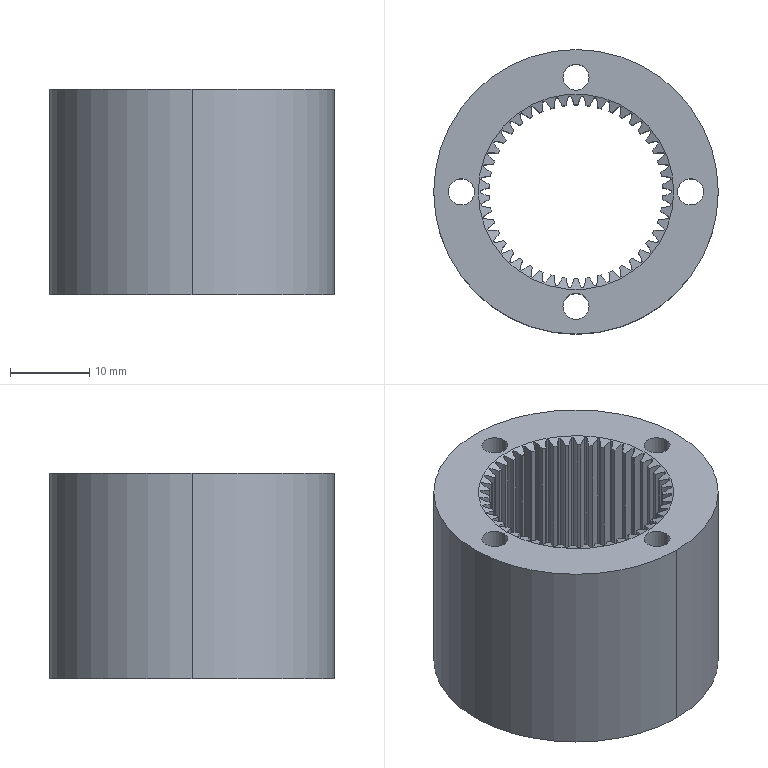Part | SolidWorks | features BaseBody 1 | 1 solid | 202 faces | box 36 x 36 x 26 mm | volume 14714 mm3 | cylinder 104 | spline 92 | cone 4 | plane 2 | commonest cylinder face diameters 24.25 x47 21.991 x46 3.3 x8 36 x3